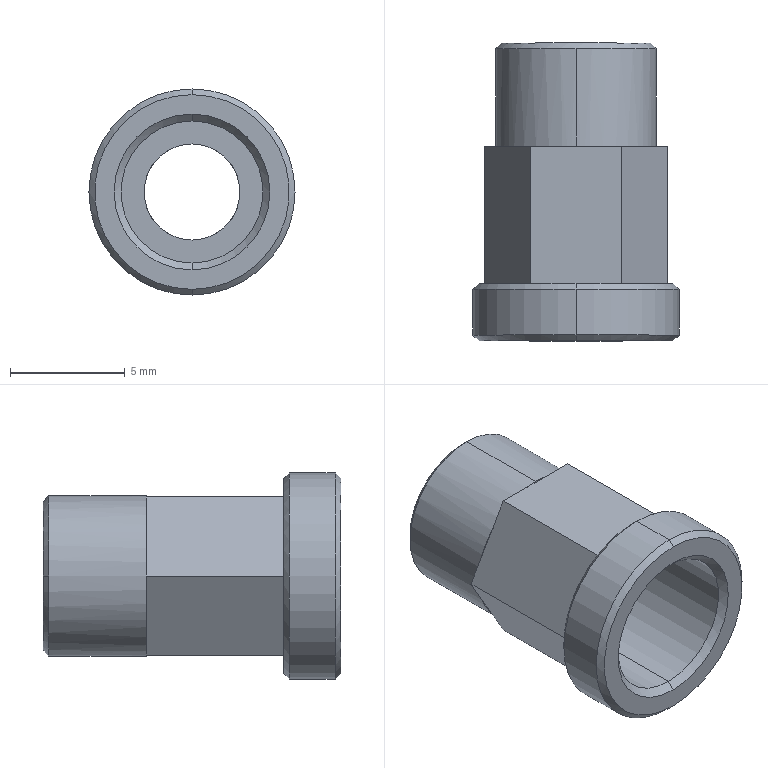Part | NX | features BREP 1 | 1 solid | 40 faces | box 9 x 13 x 9 mm | volume 256.908 mm3 | plane 22 | cone 10 | cylinder 8 | commonest cylinder face diameters 4.2 x2 6.2 x2 7 x2 9 x2
STEP:
#1=CARTESIAN_POINT('',(0.,8.5,3.1));
#2=VERTEX_POINT('',#1);
#3=CARTESIAN_POINT('',(0.,8.5,-3.1));
#4=VERTEX_POINT('',#3);
#5=CARTESIAN_POINT('',(0.,8.5,0.));
#6=DIRECTION('',(0.,-1.,0.));
#7=DIRECTION('',(0.,0.,-1.));
#8=AXIS2_PLACEMENT_3D('',#5,#6,#7);
#9=CIRCLE('',#8,3.1);
#10=EDGE_CURVE('',#2,#4,#9,.T.);
#11=ORIENTED_EDGE('',*,*,#10,.F.);
#12=CARTESIAN_POINT('',(0.,0.3,3.1));
#13=VERTEX_POINT('',#12);
#14=CARTESIAN_POINT('',(0.,0.,3.1));
#15=DIRECTION('',(0.,-1.,0.));
#16=VECTOR('',#15,1000.);
#17=LINE('',#14,#16);
#18=EDGE_CURVE('',#13,#2,#17,.F.);
#19=ORIENTED_EDGE('',*,*,#18,.F.);
#20=CARTESIAN_POINT('',(0.,0.3,-3.1));
#21=VERTEX_POINT('',#20);
#22=CARTESIAN_POINT('',(0.,0.3,0.));
#23=DIRECTION('',(0.,1.,0.));
#24=DIRECTION('',(0.,0.,-1.));
#25=AXIS2_PLACEMENT_3D('',#22,#23,#24);
#26=CIRCLE('',#25,3.1);
#27=EDGE_CURVE('',#21,#13,#26,.T.);
#28=ORIENTED_EDGE('',*,*,#27,.F.);
#29=CARTESIAN_POINT('',(0.,0.,-3.1));
#30=DIRECTION('',(0.,-1.,0.));
#31=VECTOR('',#30,1000.);
#32=LINE('',#29,#31);
#33=EDGE_CURVE('',#21,#4,#32,.F.);
#34=ORIENTED_EDGE('',*,*,#33,.T.);
#35=EDGE_LOOP('',(#11,#19,#28,#34));
#36=FACE_BOUND('',#35,.T.);
#37=CARTESIAN_POINT('',(0.,0.,0.));
#38=DIRECTION('',(0.,-1.,0.));
#39=DIRECTION('',(0.,0.,1.));
#40=AXIS2_PLACEMENT_3D('',#37,#38,#39);
#41=CYLINDRICAL_SURFACE('',#40,3.1);
#42=ADVANCED_FACE('',(#36),#41,.F.);
#43=ORIENTED_EDGE('',*,*,#27,.T.);
#44=CARTESIAN_POINT('',(0.,0.,3.4));
#45=VERTEX_POINT('',#44);
#46=CARTESIAN_POINT('',(0.,0.,3.4));
#47=DIRECTION('',(0.,-0.7071,0.7071));
#48=VECTOR('',#47,1000.);
#49=LINE('',#46,#48);
#50=EDGE_CURVE('',#45,#13,#49,.F.);
#51=ORIENTED_EDGE('',*,*,#50,.F.);
#52=CARTESIAN_POINT('',(0.,0.,-3.4));
#53=VERTEX_POINT('',#52);
#54=CARTESIAN_POINT('',(0.,0.,0.));
#55=DIRECTION('',(0.,1.,0.));
#56=DIRECTION('',(0.,0.,-1.));
#57=AXIS2_PLACEMENT_3D('',#54,#55,#56);
#58=CIRCLE('',#57,3.4);
#59=EDGE_CURVE('',#53,#45,#58,.T.);
#60=ORIENTED_EDGE('',*,*,#59,.F.);
#61=CARTESIAN_POINT('',(0.,0.,-3.4));
#62=DIRECTION('',(0.,-0.7071,-0.7071));
#63=VECTOR('',#62,1000.);
#64=LINE('',#61,#63);
#65=EDGE_CURVE('',#53,#21,#64,.F.);
#66=ORIENTED_EDGE('',*,*,#65,.T.);
#67=EDGE_LOOP('',(#43,#51,#60,#66));
#68=FACE_BOUND('',#67,.T.);
#69=CARTESIAN_POINT('',(0.,0.,0.));
#70=DIRECTION('',(0.,-1.,0.));
#71=DIRECTION('',(0.,0.,1.));
#72=AXIS2_PLACEMENT_3D('',#69,#70,#71);
#73=CONICAL_SURFACE('',#72,3.4,0.7854);
#74=ADVANCED_FACE('',(#68),#73,.F.);
#75=CARTESIAN_POINT('',(0.,8.5,2.1));
#76=VERTEX_POINT('',#75);
#77=CARTESIAN_POINT('',(0.,8.5,-2.1));
#78=VERTEX_POINT('',#77);
#79=CARTESIAN_POINT('',(0.,8.5,0.));
#80=DIRECTION('',(0.,-1.,0.));
#81=DIRECTION('',(0.,0.,1.));
#82=AXIS2_PLACEMENT_3D('',#79,#80,#81);
#83=CIRCLE('',#82,2.1);
#84=EDGE_CURVE('',#76,#78,#83,.T.);
#85=ORIENTED_EDGE('',*,*,#84,.T.);
#86=CARTESIAN_POINT('',(0.,12.75,-2.1));
#87=VERTEX_POINT('',#86);
#88=CARTESIAN_POINT('',(0.,6.95,-2.1));
#89=DIRECTION('',(0.,1.,0.));
#90=VECTOR('',#89,1000.);
#91=LINE('',#88,#90);
#92=EDGE_CURVE('',#78,#87,#91,.T.);
#93=ORIENTED_EDGE('',*,*,#92,.T.);
#94=CARTESIAN_POINT('',(-2.1,12.75,0.));
#95=VERTEX_POINT('',#94);
#96=CARTESIAN_POINT('',(0.,12.75,0.));
#97=DIRECTION('',(0.,-1.,0.));
#98=DIRECTION('',(0.,0.,1.));
#99=AXIS2_PLACEMENT_3D('',#96,#97,#98);
#100=CIRCLE('',#99,2.1);
#101=EDGE_CURVE('',#95,#87,#100,.T.);
#102=ORIENTED_EDGE('',*,*,#101,.F.);
#103=CARTESIAN_POINT('',(0.,12.75,2.1));
#104=VERTEX_POINT('',#103);
#105=CARTESIAN_POINT('',(0.,12.75,0.));
#106=DIRECTION('',(0.,-1.,0.));
#107=DIRECTION('',(0.,0.,1.));
#108=AXIS2_PLACEMENT_3D('',#105,#106,#107);
#109=CIRCLE('',#108,2.1);
#110=EDGE_CURVE('',#104,#95,#109,.T.);
#111=ORIENTED_EDGE('',*,*,#110,.F.);
#112=CARTESIAN_POINT('',(0.,6.95,2.1));
#113=DIRECTION('',(0.,1.,0.));
#114=VECTOR('',#113,1000.);
#115=LINE('',#112,#114);
#116=EDGE_CURVE('',#76,#104,#115,.T.);
#117=ORIENTED_EDGE('',*,*,#116,.F.);
#118=EDGE_LOOP('',(#85,#93,#102,#111,#117));
#119=FACE_BOUND('',#118,.T.);
#120=CARTESIAN_POINT('',(0.,6.95,0.));
#121=DIRECTION('',(0.,1.,0.));
#122=DIRECTION('',(0.,0.,-1.));
#123=AXIS2_PLACEMENT_3D('',#120,#121,#122);
#124=CYLINDRICAL_SURFACE('',#123,2.1);
#125=ADVANCED_FACE('',(#119),#124,.F.);
#126=ORIENTED_EDGE('',*,*,#101,.T.);
#127=CARTESIAN_POINT('',(2.1,12.75,0.));
#128=VERTEX_POINT('',#127);
#129=CARTESIAN_POINT('',(0.,12.75,0.));
#130=DIRECTION('',(0.,-1.,0.));
#131=DIRECTION('',(0.,0.,1.));
#132=AXIS2_PLACEMENT_3D('',#129,#130,#131);
#133=CIRCLE('',#132,2.1);
#134=EDGE_CURVE('',#87,#128,#133,.T.);
#135=ORIENTED_EDGE('',*,*,#134,.T.);
#136=CARTESIAN_POINT('',(2.35,13.,0.));
#137=VERTEX_POINT('',#136);
#138=CARTESIAN_POINT('',(2.35,13.,0.));
#139=DIRECTION('',(0.7071,0.7071,0.));
#140=VECTOR('',#139,1000.);
#141=LINE('',#138,#140);
#142=EDGE_CURVE('',#137,#128,#141,.F.);
#143=ORIENTED_EDGE('',*,*,#142,.F.);
#144=CARTESIAN_POINT('',(-2.35,13.,0.));
#145=VERTEX_POINT('',#144);
#146=CARTESIAN_POINT('',(0.,13.,0.));
#147=DIRECTION('',(0.,-1.,0.));
#148=DIRECTION('',(-1.,0.,0.));
#149=AXIS2_PLACEMENT_3D('',#146,#147,#148);
#150=CIRCLE('',#149,2.35);
#151=EDGE_CURVE('',#145,#137,#150,.T.);
#152=ORIENTED_EDGE('',*,*,#151,.F.);
#153=CARTESIAN_POINT('',(-2.35,13.,0.));
#154=DIRECTION('',(-0.7071,0.7071,0.));
#155=VECTOR('',#154,1000.);
#156=LINE('',#153,#155);
#157=EDGE_CURVE('',#145,#95,#156,.F.);
#158=ORIENTED_EDGE('',*,*,#157,.T.);
#159=EDGE_LOOP('',(#126,#135,#143,#152,#158));
#160=FACE_BOUND('',#159,.T.);
#161=CARTESIAN_POINT('',(0.,13.,0.));
#162=DIRECTION('',(0.,1.,0.));
#163=DIRECTION('',(1.,0.,0.));
#164=AXIS2_PLACEMENT_3D('',#161,#162,#163);
#165=CONICAL_SURFACE('',#164,2.35,0.7854);
#166=ADVANCED_FACE('',(#160),#165,.F.);
#167=CARTESIAN_POINT('',(0.,-0.000000001,-4.25));
#168=VERTEX_POINT('',#167);
#169=CARTESIAN_POINT('',(0.,-0.000000001,4.25));
#170=VERTEX_POINT('',#169);
#171=CARTESIAN_POINT('',(0.,-0.000000001,0.));
#172=DIRECTION('',(0.,-1.,0.));
#173=DIRECTION('',(0.,0.,1.));
#174=AXIS2_PLACEMENT_3D('',#171,#172,#173);
#175=CIRCLE('',#174,4.25);
#176=EDGE_CURVE('',#168,#170,#175,.T.);
#177=ORIENTED_EDGE('',*,*,#176,.F.);
#178=CARTESIAN_POINT('',(0.,0.25,-4.5));
#179=VERTEX_POINT('',#178);
#180=CARTESIAN_POINT('',(0.,0.25,-4.5));
#181=DIRECTION('',(0.,0.7071,-0.7071));
#182=VECTOR('',#181,1000.);
#183=LINE('',#180,#182);
#184=EDGE_CURVE('',#168,#179,#183,.T.);
#185=ORIENTED_EDGE('',*,*,#184,.T.);
#186=CARTESIAN_POINT('',(0.,0.25,4.5));
#187=VERTEX_POINT('',#186);
#188=CARTESIAN_POINT('',(0.,0.25,0.));
#189=DIRECTION('',(0.,-1.,0.));
#190=DIRECTION('',(0.,0.,1.));
#191=AXIS2_PLACEMENT_3D('',#188,#189,#190);
#192=CIRCLE('',#191,4.5);
#193=EDGE_CURVE('',#179,#187,#192,.T.);
#194=ORIENTED_EDGE('',*,*,#193,.T.);
#195=CARTESIAN_POINT('',(0.,0.25,4.5));
#196=DIRECTION('',(0.,0.7071,0.7071));
#197=VECTOR('',#196,1000.);
#198=LINE('',#195,#197);
#199=EDGE_CURVE('',#170,#187,#198,.T.);
#200=ORIENTED_EDGE('',*,*,#199,.F.);
#201=EDGE_LOOP('',(#177,#185,#194,#200));
#202=FACE_BOUND('',#201,.T.);
#203=CARTESIAN_POINT('',(0.,0.25,0.));
#204=DIRECTION('',(0.,1.,0.));
#205=DIRECTION('',(0.,0.,-1.));
#206=AXIS2_PLACEMENT_3D('',#203,#204,#205);
#207=CONICAL_SURFACE('',#206,4.5,0.7854);
#208=ADVANCED_FACE('',(#202),#207,.T.);
#209=CARTESIAN_POINT('',(0.,2.25,-4.5));
#210=VERTEX_POINT('',#209);
#211=CARTESIAN_POINT('',(0.,2.25,4.5));
#212=VERTEX_POINT('',#211);
#213=CARTESIAN_POINT('',(0.,2.25,0.));
#214=DIRECTION('',(0.,-1.,0.));
#215=DIRECTION('',(0.,0.,-1.));
#216=AXIS2_PLACEMENT_3D('',#213,#214,#215);
#217=CIRCLE('',#216,4.5);
#218=EDGE_CURVE('',#210,#212,#217,.T.);
#219=ORIENTED_EDGE('',*,*,#218,.T.);
#220=CARTESIAN_POINT('',(0.,0.5,4.5));
#221=DIRECTION('',(0.,-1.,0.));
#222=VECTOR('',#221,1000.);
#223=LINE('',#220,#222);
#224=EDGE_CURVE('',#187,#212,#223,.F.);
#225=ORIENTED_EDGE('',*,*,#224,.F.);
#226=ORIENTED_EDGE('',*,*,#193,.F.);
#227=CARTESIAN_POINT('',(0.,0.5,-4.5));
#228=DIRECTION('',(0.,-1.,0.));
#229=VECTOR('',#228,1000.);
#230=LINE('',#227,#229);
#231=EDGE_CURVE('',#179,#210,#230,.F.);
#232=ORIENTED_EDGE('',*,*,#231,.T.);
#233=EDGE_LOOP('',(#219,#225,#226,#232));
#234=FACE_BOUND('',#233,.T.);
#235=CARTESIAN_POINT('',(0.,0.5,0.));
#236=DIRECTION('',(0.,-1.,0.));
#237=DIRECTION('',(0.,0.,1.));
#238=AXIS2_PLACEMENT_3D('',#235,#236,#237);
#239=CYLINDRICAL_SURFACE('',#238,4.5);
#240=ADVANCED_FACE('',(#234),#239,.T.);
#241=CARTESIAN_POINT('',(-3.25,13.,0.));
#242=VERTEX_POINT('',#241);
#243=CARTESIAN_POINT('',(3.25,13.,0.));
#244=VERTEX_POINT('',#243);
#245=CARTESIAN_POINT('',(0.,13.,0.));
#246=DIRECTION('',(0.,1.,0.));
#247=DIRECTION('',(1.,0.,0.));
#248=AXIS2_PLACEMENT_3D('',#245,#246,#247);
#249=CIRCLE('',#248,3.25);
#250=EDGE_CURVE('',#242,#244,#249,.T.);
#251=ORIENTED_EDGE('',*,*,#250,.F.);
#252=CARTESIAN_POINT('',(-3.5,12.75,0.));
#253=VERTEX_POINT('',#252);
#254=CARTESIAN_POINT('',(-3.5,12.75,0.));
#255=DIRECTION('',(-0.7071,-0.7071,0.));
#256=VECTOR('',#255,1000.);
#257=LINE('',#254,#256);
#258=EDGE_CURVE('',#242,#253,#257,.T.);
#259=ORIENTED_EDGE('',*,*,#258,.T.);
#260=CARTESIAN_POINT('',(0.,12.75,3.5));
#261=VERTEX_POINT('',#260);
#262=CARTESIAN_POINT('',(0.,12.75,0.));
#263=DIRECTION('',(0.,1.,0.));
#264=DIRECTION('',(0.,0.,-1.));
#265=AXIS2_PLACEMENT_3D('',#262,#263,#264);
#266=CIRCLE('',#265,3.5);
#267=EDGE_CURVE('',#253,#261,#266,.T.);
#268=ORIENTED_EDGE('',*,*,#267,.T.);
#269=CARTESIAN_POINT('',(3.5,12.75,0.));
#270=VERTEX_POINT('',#269);
#271=CARTESIAN_POINT('',(0.,12.75,0.));
#272=DIRECTION('',(0.,1.,0.));
#273=DIRECTION('',(0.,0.,-1.));
#274=AXIS2_PLACEMENT_3D('',#271,#272,#273);
#275=CIRCLE('',#274,3.5);
#276=EDGE_CURVE('',#261,#270,#275,.T.);
#277=ORIENTED_EDGE('',*,*,#276,.T.);
#278=CARTESIAN_POINT('',(3.5,12.75,0.));
#279=DIRECTION('',(0.7071,-0.7071,0.));
#280=VECTOR('',#279,1000.);
#281=LINE('',#278,#280);
#282=EDGE_CURVE('',#244,#270,#281,.T.);
#283=ORIENTED_EDGE('',*,*,#282,.F.);
#284=EDGE_LOOP('',(#251,#259,#268,#277,#283));
#285=FACE_BOUND('',#284,.T.);
#286=CARTESIAN_POINT('',(0.,12.75,0.));
#287=DIRECTION('',(0.,-1.,0.));
#288=DIRECTION('',(-1.,0.,0.));
#289=AXIS2_PLACEMENT_3D('',#286,#287,#288);
#290=CONICAL_SURFACE('',#289,3.5,0.7854);
#291=ADVANCED_FACE('',(#285),#290,.T.);
#292=CARTESIAN_POINT('',(0.,2.5,-4.25));
#293=VERTEX_POINT('',#292);
#294=CARTESIAN_POINT('',(0.,2.5,4.25));
#295=VERTEX_POINT('',#294);
#296=CARTESIAN_POINT('',(0.,2.5,0.));
#297=DIRECTION('',(0.,-1.,0.));
#298=DIRECTION('',(0.,0.,-1.));
#299=AXIS2_PLACEMENT_3D('',#296,#297,#298);
#300=CIRCLE('',#299,4.25);
#301=EDGE_CURVE('',#293,#295,#300,.T.);
#302=ORIENTED_EDGE('',*,*,#301,.T.);
#303=CARTESIAN_POINT('',(0.,2.25,4.5));
#304=DIRECTION('',(0.,-0.7071,0.7071));
#305=VECTOR('',#304,1000.);
#306=LINE('',#303,#305);
#307=EDGE_CURVE('',#212,#295,#306,.F.);
#308=ORIENTED_EDGE('',*,*,#307,.F.);
#309=ORIENTED_EDGE('',*,*,#218,.F.);
#310=CARTESIAN_POINT('',(0.,2.25,-4.5));
#311=DIRECTION('',(0.,-0.7071,-0.7071));
#312=VECTOR('',#311,1000.);
#313=LINE('',#310,#312);
#314=EDGE_CURVE('',#210,#293,#313,.F.);
#315=ORIENTED_EDGE('',*,*,#314,.T.);
#316=EDGE_LOOP('',(#302,#308,#309,#315));
#317=FACE_BOUND('',#316,.T.);
#318=CARTESIAN_POINT('',(0.,2.25,0.));
#319=DIRECTION('',(0.,-1.,0.));
#320=DIRECTION('',(0.,0.,1.));
#321=AXIS2_PLACEMENT_3D('',#318,#319,#320);
#322=CONICAL_SURFACE('',#321,4.5,0.7854);
#323=ADVANCED_FACE('',(#317),#322,.T.);
#324=CARTESIAN_POINT('',(0.5895,8.5,-3.45));
#325=VERTEX_POINT('',#324);
#326=CARTESIAN_POINT('',(0.,8.5,-3.5));
#327=VERTEX_POINT('',#326);
#328=CARTESIAN_POINT('',(0.,8.5,0.));
#329=DIRECTION('',(0.,1.,0.));
#330=DIRECTION('',(0.,0.,1.));
#331=AXIS2_PLACEMENT_3D('',#328,#329,#330);
#332=CIRCLE('',#331,3.5);
#333=EDGE_CURVE('',#325,#327,#332,.T.);
#334=ORIENTED_EDGE('',*,*,#333,.T.);
#335=CARTESIAN_POINT('',(0.,12.75,-3.5));
#336=VERTEX_POINT('',#335);
#337=CARTESIAN_POINT('',(0.,8.5,-3.5));
#338=DIRECTION('',(0.,1.,0.));
#339=VECTOR('',#338,1000.);
#340=LINE('',#337,#339);
#341=EDGE_CURVE('',#327,#336,#340,.T.);
#342=ORIENTED_EDGE('',*,*,#341,.T.);
#343=CARTESIAN_POINT('',(0.,12.75,0.));
#344=DIRECTION('',(0.,1.,0.));
#345=DIRECTION('',(0.,0.,-1.));
#346=AXIS2_PLACEMENT_3D('',#343,#344,#345);
#347=CIRCLE('',#346,3.5);
#348=EDGE_CURVE('',#270,#336,#347,.T.);
#349=ORIENTED_EDGE('',*,*,#348,.F.);
#350=ORIENTED_EDGE('',*,*,#276,.F.);
#351=CARTESIAN_POINT('',(0.,8.5,3.5));
#352=VERTEX_POINT('',#351);
#353=CARTESIAN_POINT('',(0.,8.5,3.5));
#354=DIRECTION('',(0.,1.,0.));
#355=VECTOR('',#354,1000.);
#356=LINE('',#353,#355);
#357=EDGE_CURVE('',#352,#261,#356,.T.);
#358=ORIENTED_EDGE('',*,*,#357,.F.);
#359=CARTESIAN_POINT('',(0.5895,8.5,3.45));
#360=VERTEX_POINT('',#359);
#361=CARTESIAN_POINT('',(0.,8.5,0.));
#362=DIRECTION('',(0.,1.,0.));
#363=DIRECTION('',(0.,0.,1.));
#364=AXIS2_PLACEMENT_3D('',#361,#362,#363);
#365=CIRCLE('',#364,3.5);
#366=EDGE_CURVE('',#352,#360,#365,.T.);
#367=ORIENTED_EDGE('',*,*,#366,.T.);
#368=CARTESIAN_POINT('',(2.693,8.5,2.236));
#369=VERTEX_POINT('',#368);
#370=CARTESIAN_POINT('',(0.,8.5,0.));
#371=DIRECTION('',(0.,1.,0.));
#372=DIRECTION('',(0.,0.,1.));
#373=AXIS2_PLACEMENT_3D('',#370,#371,#372);
#374=CIRCLE('',#373,3.5);
#375=EDGE_CURVE('',#360,#369,#374,.T.);
#376=ORIENTED_EDGE('',*,*,#375,.T.);
#377=CARTESIAN_POINT('',(3.283,8.5,1.214));
#378=VERTEX_POINT('',#377);
#379=CARTESIAN_POINT('',(0.,8.5,0.));
#380=DIRECTION('',(0.,1.,0.));
#381=DIRECTION('',(0.,0.,1.));
#382=AXIS2_PLACEMENT_3D('',#379,#380,#381);
#383=CIRCLE('',#382,3.5);
#384=EDGE_CURVE('',#369,#378,#383,.T.);
#385=ORIENTED_EDGE('',*,*,#384,.T.);
#386=CARTESIAN_POINT('',(3.283,8.5,-1.214));
#387=VERTEX_POINT('',#386);
#388=CARTESIAN_POINT('',(0.,8.5,0.));
#389=DIRECTION('',(0.,1.,0.));
#390=DIRECTION('',(0.,0.,1.));
#391=AXIS2_PLACEMENT_3D('',#388,#389,#390);
#392=CIRCLE('',#391,3.5);
#393=EDGE_CURVE('',#378,#387,#392,.T.);
#394=ORIENTED_EDGE('',*,*,#393,.T.);
#395=CARTESIAN_POINT('',(2.693,8.5,-2.236));
#396=VERTEX_POINT('',#395);
#397=CARTESIAN_POINT('',(0.,8.5,0.));
#398=DIRECTION('',(0.,1.,0.));
#399=DIRECTION('',(0.,0.,1.));
#400=AXIS2_PLACEMENT_3D('',#397,#398,#399);
#401=CIRCLE('',#400,3.5);
#402=EDGE_CURVE('',#387,#396,#401,.T.);
#403=ORIENTED_EDGE('',*,*,#402,.T.);
#404=CARTESIAN_POINT('',(0.,8.5,0.));
#405=DIRECTION('',(0.,1.,0.));
#406=DIRECTION('',(0.,0.,1.));
#407=AXIS2_PLACEMENT_3D('',#404,#405,#406);
#408=CIRCLE('',#407,3.5);
#409=EDGE_CURVE('',#396,#325,#408,.T.);
#410=ORIENTED_EDGE('',*,*,#409,.T.);
#411=EDGE_LOOP('',(#334,#342,#349,#350,#358,#367,#376,#385,#394,#403,#410));
#412=FACE_BOUND('',#411,.T.);
#413=CARTESIAN_POINT('',(0.,8.5,0.));
#414=DIRECTION('',(0.,1.,0.));
#415=DIRECTION('',(0.,0.,-1.));
#416=AXIS2_PLACEMENT_3D('',#413,#414,#415);
#417=CYLINDRICAL_SURFACE('',#416,3.5);
#418=ADVANCED_FACE('',(#412),#417,.T.);
#419=ORIENTED_EDGE('',*,*,#18,.T.);
#420=CARTESIAN_POINT('',(0.,8.5,0.));
#421=DIRECTION('',(0.,-1.,0.));
#422=DIRECTION('',(0.,0.,-1.));
#423=AXIS2_PLACEMENT_3D('',#420,#421,#422);
#424=CIRCLE('',#423,3.1);
#425=EDGE_CURVE('',#4,#2,#424,.T.);
#426=ORIENTED_EDGE('',*,*,#425,.F.);
#427=ORIENTED_EDGE('',*,*,#33,.F.);
#428=CARTESIAN_POINT('',(0.,0.3,0.));
#429=DIRECTION('',(0.,1.,0.));
#430=DIRECTION('',(0.,0.,-1.));
#431=AXIS2_PLACEMENT_3D('',#428,#429,#430);
#432=CIRCLE('',#431,3.1);
#433=EDGE_CURVE('',#13,#21,#432,.T.);
#434=ORIENTED_EDGE('',*,*,#433,.F.);
#435=EDGE_LOOP('',(#419,#426,#427,#434));
#436=FACE_BOUND('',#435,.T.);
#437=CARTESIAN_POINT('',(0.,0.,0.));
#438=DIRECTION('',(0.,-1.,0.));
#439=DIRECTION('',(0.,0.,1.));
#440=AXIS2_PLACEMENT_3D('',#437,#438,#439);
#441=CYLINDRICAL_SURFACE('',#440,3.1);
#442=ADVANCED_FACE('',(#436),#441,.F.);
#443=ORIENTED_EDGE('',*,*,#425,.T.);
#444=ORIENTED_EDGE('',*,*,#10,.T.);
#445=EDGE_LOOP('',(#443,#444));
#446=FACE_BOUND('',#445,.T.);
#447=ORIENTED_EDGE('',*,*,#84,.F.);
#448=CARTESIAN_POINT('',(0.,8.5,0.));
#449=DIRECTION('',(0.,-1.,0.));
#450=DIRECTION('',(0.,0.,1.));
#451=AXIS2_PLACEMENT_3D('',#448,#449,#450);
#452=CIRCLE('',#451,2.1);
#453=EDGE_CURVE('',#78,#76,#452,.T.);
#454=ORIENTED_EDGE('',*,*,#453,.F.);
#455=EDGE_LOOP('',(#447,#454));
#456=FACE_BOUND('',#455,.T.);
#457=CARTESIAN_POINT('',(0.,8.5,0.));
#458=DIRECTION('',(0.,1.,0.));
#459=DIRECTION('',(0.,0.,-1.));
#460=AXIS2_PLACEMENT_3D('',#457,#458,#459);
#461=PLANE('',#460);
#462=ADVANCED_FACE('',(#446,#456),#461,.F.);
#463=ORIENTED_EDGE('',*,*,#50,.T.);
#464=ORIENTED_EDGE('',*,*,#433,.T.);
#465=ORIENTED_EDGE('',*,*,#65,.F.);
#466=CARTESIAN_POINT('',(0.,0.,0.));
#467=DIRECTION('',(0.,1.,0.));
#468=DIRECTION('',(0.,0.,-1.));
#469=AXIS2_PLACEMENT_3D('',#466,#467,#468);
#470=CIRCLE('',#469,3.4);
#471=EDGE_CURVE('',#45,#53,#470,.T.);
#472=ORIENTED_EDGE('',*,*,#471,.F.);
#473=EDGE_LOOP('',(#463,#464,#465,#472));
#474=FACE_BOUND('',#473,.T.);
#475=CARTESIAN_POINT('',(0.,0.,0.));
#476=DIRECTION('',(0.,-1.,0.));
#477=DIRECTION('',(0.,0.,1.));
#478=AXIS2_PLACEMENT_3D('',#475,#476,#477);
#479=CONICAL_SURFACE('',#478,3.4,0.7854);
#480=ADVANCED_FACE('',(#474),#479,.F.);
#481=ORIENTED_EDGE('',*,*,#92,.F.);
#482=ORIENTED_EDGE('',*,*,#453,.T.);
#483=ORIENTED_EDGE('',*,*,#116,.T.);
#484=CARTESIAN_POINT('',(0.,12.75,0.));
#485=DIRECTION('',(0.,-1.,0.));
#486=DIRECTION('',(0.,0.,1.));
#487=AXIS2_PLACEMENT_3D('',#484,#485,#486);
#488=CIRCLE('',#487,2.1);
#489=EDGE_CURVE('',#128,#104,#488,.T.);
#490=ORIENTED_EDGE('',*,*,#489,.F.);
#491=ORIENTED_EDGE('',*,*,#134,.F.);
#492=EDGE_LOOP('',(#481,#482,#483,#490,#491));
#493=FACE_BOUND('',#492,.T.);
#494=CARTESIAN_POINT('',(0.,6.95,0.));
#495=DIRECTION('',(0.,1.,0.));
#496=DIRECTION('',(0.,0.,-1.));
#497=AXIS2_PLACEMENT_3D('',#494,#495,#496);
#498=CYLINDRICAL_SURFACE('',#497,2.1);
#499=ADVANCED_FACE('',(#493),#498,.F.);
#500=CARTESIAN_POINT('',(0.,-0.000000001,0.));
#501=DIRECTION('',(0.,-1.,0.));
#502=DIRECTION('',(0.,0.,1.));
#503=AXIS2_PLACEMENT_3D('',#500,#501,#502);
#504=CIRCLE('',#503,4.25);
#505=EDGE_CURVE('',#170,#168,#504,.T.);
#506=ORIENTED_EDGE('',*,*,#505,.T.);
#507=ORIENTED_EDGE('',*,*,#176,.T.);
#508=EDGE_LOOP('',(#506,#507));
#509=FACE_BOUND('',#508,.T.);
#510=ORIENTED_EDGE('',*,*,#59,.T.);
#511=ORIENTED_EDGE('',*,*,#471,.T.);
#512=EDGE_LOOP('',(#510,#511));
#513=FACE_BOUND('',#512,.T.);
#514=CARTESIAN_POINT('',(0.,0.,0.));
#515=DIRECTION('',(0.,-1.,0.));
#516=DIRECTION('',(0.,0.,1.));
#517=AXIS2_PLACEMENT_3D('',#514,#515,#516);
#518=PLANE('',#517);
#519=ADVANCED_FACE('',(#509,#513),#518,.T.);
#520=ORIENTED_EDGE('',*,*,#142,.T.);
#521=ORIENTED_EDGE('',*,*,#489,.T.);
#522=ORIENTED_EDGE('',*,*,#110,.T.);
#523=ORIENTED_EDGE('',*,*,#157,.F.);
#524=CARTESIAN_POINT('',(0.,13.,0.));
#525=DIRECTION('',(0.,-1.,0.));
#526=DIRECTION('',(-1.,0.,0.));
#527=AXIS2_PLACEMENT_3D('',#524,#525,#526);
#528=CIRCLE('',#527,2.35);
#529=EDGE_CURVE('',#137,#145,#528,.T.);
#530=ORIENTED_EDGE('',*,*,#529,.F.);
#531=EDGE_LOOP('',(#520,#521,#522,#523,#530));
#532=FACE_BOUND('',#531,.T.);
#533=CARTESIAN_POINT('',(0.,13.,0.));
#534=DIRECTION('',(0.,1.,0.));
#535=DIRECTION('',(1.,0.,0.));
#536=AXIS2_PLACEMENT_3D('',#533,#534,#535);
#537=CONICAL_SURFACE('',#536,2.35,0.7854);
#538=ADVANCED_FACE('',(#532),#537,.F.);
#539=ORIENTED_EDGE('',*,*,#184,.F.);
#540=ORIENTED_EDGE('',*,*,#505,.F.);
#541=ORIENTED_EDGE('',*,*,#199,.T.);
#542=CARTESIAN_POINT('',(0.,0.25,0.));
#543=DIRECTION('',(0.,-1.,0.));
#544=DIRECTION('',(0.,0.,1.));
#545=AXIS2_PLACEMENT_3D('',#542,#543,#544);
#546=CIRCLE('',#545,4.5);
#547=EDGE_CURVE('',#187,#179,#546,.T.);
#548=ORIENTED_EDGE('',*,*,#547,.T.);
#549=EDGE_LOOP('',(#539,#540,#541,#548));
#550=FACE_BOUND('',#549,.T.);
#551=CARTESIAN_POINT('',(0.,0.25,0.));
#552=DIRECTION('',(0.,1.,0.));
#553=DIRECTION('',(0.,0.,-1.));
#554=AXIS2_PLACEMENT_3D('',#551,#552,#553);
#555=CONICAL_SURFACE('',#554,4.5,0.7854);
#556=ADVANCED_FACE('',(#550),#555,.T.);
#557=CARTESIAN_POINT('',(0.,13.,0.));
#558=DIRECTION('',(0.,1.,0.));
#559=DIRECTION('',(1.,0.,0.));
#560=AXIS2_PLACEMENT_3D('',#557,#558,#559);
#561=CIRCLE('',#560,3.25);
#562=EDGE_CURVE('',#244,#242,#561,.T.);
#563=ORIENTED_EDGE('',*,*,#562,.T.);
#564=ORIENTED_EDGE('',*,*,#250,.T.);
#565=EDGE_LOOP('',(#563,#564));
#566=FACE_BOUND('',#565,.T.);
#567=ORIENTED_EDGE('',*,*,#151,.T.);
#568=ORIENTED_EDGE('',*,*,#529,.T.);
#569=EDGE_LOOP('',(#567,#568));
#570=FACE_BOUND('',#569,.T.);
#571=CARTESIAN_POINT('',(0.,13.,0.));
#572=DIRECTION('',(0.,1.,0.));
#573=DIRECTION('',(0.,0.,-1.));
#574=AXIS2_PLACEMENT_3D('',#571,#572,#573);
#575=PLANE('',#574);
#576=ADVANCED_FACE('',(#566,#570),#575,.T.);
#577=ORIENTED_EDGE('',*,*,#224,.T.);
#578=CARTESIAN_POINT('',(0.,2.25,0.));
#579=DIRECTION('',(0.,-1.,0.));
#580=DIRECTION('',(0.,0.,-1.));
#581=AXIS2_PLACEMENT_3D('',#578,#579,#580);
#582=CIRCLE('',#581,4.5);
#583=EDGE_CURVE('',#212,#210,#582,.T.);
#584=ORIENTED_EDGE('',*,*,#583,.T.);
#585=ORIENTED_EDGE('',*,*,#231,.F.);
#586=ORIENTED_EDGE('',*,*,#547,.F.);
#587=EDGE_LOOP('',(#577,#584,#585,#586));
#588=FACE_BOUND('',#587,.T.);
#589=CARTESIAN_POINT('',(0.,0.5,0.));
#590=DIRECTION('',(0.,-1.,0.));
#591=DIRECTION('',(0.,0.,1.));
#592=AXIS2_PLACEMENT_3D('',#589,#590,#591);
#593=CYLINDRICAL_SURFACE('',#592,4.5);
#594=ADVANCED_FACE('',(#588),#593,.T.);
#595=ORIENTED_EDGE('',*,*,#258,.F.);
#596=ORIENTED_EDGE('',*,*,#562,.F.);
#597=ORIENTED_EDGE('',*,*,#282,.T.);
#598=ORIENTED_EDGE('',*,*,#348,.T.);
#599=CARTESIAN_POINT('',(0.,12.75,0.));
#600=DIRECTION('',(0.,1.,0.));
#601=DIRECTION('',(0.,0.,-1.));
#602=AXIS2_PLACEMENT_3D('',#599,#600,#601);
#603=CIRCLE('',#602,3.5);
#604=EDGE_CURVE('',#336,#253,#603,.T.);
#605=ORIENTED_EDGE('',*,*,#604,.T.);
#606=EDGE_LOOP('',(#595,#596,#597,#598,#605));
#607=FACE_BOUND('',#606,.T.);
#608=CARTESIAN_POINT('',(0.,12.75,0.));
#609=DIRECTION('',(0.,-1.,0.));
#610=DIRECTION('',(-1.,0.,0.));
#611=AXIS2_PLACEMENT_3D('',#608,#609,#610);
#612=CONICAL_SURFACE('',#611,3.5,0.7854);
#613=ADVANCED_FACE('',(#607),#612,.T.);
#614=ORIENTED_EDGE('',*,*,#307,.T.);
#615=CARTESIAN_POINT('',(0.,2.5,0.));
#616=DIRECTION('',(0.,-1.,0.));
#617=DIRECTION('',(0.,0.,-1.));
#618=AXIS2_PLACEMENT_3D('',#615,#616,#617);
#619=CIRCLE('',#618,4.25);
#620=EDGE_CURVE('',#295,#293,#619,.T.);
#621=ORIENTED_EDGE('',*,*,#620,.T.);
#622=ORIENTED_EDGE('',*,*,#314,.F.);
#623=ORIENTED_EDGE('',*,*,#583,.F.);
#624=EDGE_LOOP('',(#614,#621,#622,#623));
#625=FACE_BOUND('',#624,.T.);
#626=CARTESIAN_POINT('',(0.,2.25,0.));
#627=DIRECTION('',(0.,-1.,0.));
#628=DIRECTION('',(0.,0.,1.));
#629=AXIS2_PLACEMENT_3D('',#626,#627,#628);
#630=CONICAL_SURFACE('',#629,4.5,0.7854);
#631=ADVANCED_FACE('',(#625),#630,.T.);
#632=ORIENTED_EDGE('',*,*,#341,.F.);
#633=CARTESIAN_POINT('',(-0.5895,8.5,-3.45));
#634=VERTEX_POINT('',#633);
#635=CARTESIAN_POINT('',(0.,8.5,0.));
#636=DIRECTION('',(0.,1.,0.));
#637=DIRECTION('',(0.,0.,1.));
#638=AXIS2_PLACEMENT_3D('',#635,#636,#637);
#639=CIRCLE('',#638,3.5);
#640=EDGE_CURVE('',#327,#634,#639,.T.);
#641=ORIENTED_EDGE('',*,*,#640,.T.);
#642=CARTESIAN_POINT('',(-2.693,8.5,-2.236));
#643=VERTEX_POINT('',#642);
#644=CARTESIAN_POINT('',(0.,8.5,0.));
#645=DIRECTION('',(0.,1.,0.));
#646=DIRECTION('',(0.,0.,1.));
#647=AXIS2_PLACEMENT_3D('',#644,#645,#646);
#648=CIRCLE('',#647,3.5);
#649=EDGE_CURVE('',#634,#643,#648,.T.);
#650=ORIENTED_EDGE('',*,*,#649,.T.);
#651=CARTESIAN_POINT('',(-3.283,8.5,-1.214));
#652=VERTEX_POINT('',#651);
#653=CARTESIAN_POINT('',(0.,8.5,0.));
#654=DIRECTION('',(0.,1.,0.));
#655=DIRECTION('',(0.,0.,1.));
#656=AXIS2_PLACEMENT_3D('',#653,#654,#655);
#657=CIRCLE('',#656,3.5);
#658=EDGE_CURVE('',#643,#652,#657,.T.);
#659=ORIENTED_EDGE('',*,*,#658,.T.);
#660=CARTESIAN_POINT('',(-3.283,8.5,1.214));
#661=VERTEX_POINT('',#660);
#662=CARTESIAN_POINT('',(0.,8.5,0.));
#663=DIRECTION('',(0.,1.,0.));
#664=DIRECTION('',(0.,0.,1.));
#665=AXIS2_PLACEMENT_3D('',#662,#663,#664);
#666=CIRCLE('',#665,3.5);
#667=EDGE_CURVE('',#652,#661,#666,.T.);
#668=ORIENTED_EDGE('',*,*,#667,.T.);
#669=CARTESIAN_POINT('',(-2.693,8.5,2.236));
#670=VERTEX_POINT('',#669);
#671=CARTESIAN_POINT('',(0.,8.5,0.));
#672=DIRECTION('',(0.,1.,0.));
#673=DIRECTION('',(0.,0.,1.));
#674=AXIS2_PLACEMENT_3D('',#671,#672,#673);
#675=CIRCLE('',#674,3.5);
#676=EDGE_CURVE('',#661,#670,#675,.T.);
#677=ORIENTED_EDGE('',*,*,#676,.T.);
#678=CARTESIAN_POINT('',(-0.5895,8.5,3.45));
#679=VERTEX_POINT('',#678);
#680=CARTESIAN_POINT('',(0.,8.5,0.));
#681=DIRECTION('',(0.,1.,0.));
#682=DIRECTION('',(0.,0.,1.));
#683=AXIS2_PLACEMENT_3D('',#680,#681,#682);
#684=CIRCLE('',#683,3.5);
#685=EDGE_CURVE('',#670,#679,#684,.T.);
#686=ORIENTED_EDGE('',*,*,#685,.T.);
#687=CARTESIAN_POINT('',(0.,8.5,0.));
#688=DIRECTION('',(0.,1.,0.));
#689=DIRECTION('',(0.,0.,1.));
#690=AXIS2_PLACEMENT_3D('',#687,#688,#689);
#691=CIRCLE('',#690,3.5);
#692=EDGE_CURVE('',#679,#352,#691,.T.);
#693=ORIENTED_EDGE('',*,*,#692,.T.);
#694=ORIENTED_EDGE('',*,*,#357,.T.);
#695=ORIENTED_EDGE('',*,*,#267,.F.);
#696=ORIENTED_EDGE('',*,*,#604,.F.);
#697=EDGE_LOOP('',(#632,#641,#650,#659,#668,#677,#686,#693,#694,#695,#696));
#698=FACE_BOUND('',#697,.T.);
#699=CARTESIAN_POINT('',(0.,8.5,0.));
#700=DIRECTION('',(0.,1.,0.));
#701=DIRECTION('',(0.,0.,-1.));
#702=AXIS2_PLACEMENT_3D('',#699,#700,#701);
#703=CYLINDRICAL_SURFACE('',#702,3.5);
#704=ADVANCED_FACE('',(#698),#703,.T.);
#705=ORIENTED_EDGE('',*,*,#301,.F.);
#706=ORIENTED_EDGE('',*,*,#620,.F.);
#707=EDGE_LOOP('',(#705,#706));
#708=FACE_BOUND('',#707,.T.);
#709=CARTESIAN_POINT('',(1.992,2.5,3.45));
#710=VERTEX_POINT('',#709);
#711=CARTESIAN_POINT('',(-1.992,2.5,3.45));
#712=VERTEX_POINT('',#711);
#713=CARTESIAN_POINT('',(0.,2.5,3.45));
#714=DIRECTION('',(-1.,0.,0.));
#715=VECTOR('',#714,1000.);
#716=LINE('',#713,#715);
#717=EDGE_CURVE('',#710,#712,#716,.T.);
#718=ORIENTED_EDGE('',*,*,#717,.T.);
#719=CARTESIAN_POINT('',(-3.984,2.5,0.));
#720=VERTEX_POINT('',#719);
#721=CARTESIAN_POINT('',(-1.992,2.5,3.45));
#722=DIRECTION('',(-0.5,0.,-0.866));
#723=VECTOR('',#722,1000.);
#724=LINE('',#721,#723);
#725=EDGE_CURVE('',#712,#720,#724,.T.);
#726=ORIENTED_EDGE('',*,*,#725,.T.);
#727=CARTESIAN_POINT('',(-1.992,2.5,-3.45));
#728=VERTEX_POINT('',#727);
#729=CARTESIAN_POINT('',(-3.984,2.5,0.));
#730=DIRECTION('',(0.5,0.,-0.866));
#731=VECTOR('',#730,1000.);
#732=LINE('',#729,#731);
#733=EDGE_CURVE('',#720,#728,#732,.T.);
#734=ORIENTED_EDGE('',*,*,#733,.T.);
#735=CARTESIAN_POINT('',(1.992,2.5,-3.45));
#736=VERTEX_POINT('',#735);
#737=CARTESIAN_POINT('',(0.,2.5,-3.45));
#738=DIRECTION('',(1.,0.,0.));
#739=VECTOR('',#738,1000.);
#740=LINE('',#737,#739);
#741=EDGE_CURVE('',#728,#736,#740,.T.);
#742=ORIENTED_EDGE('',*,*,#741,.T.);
#743=CARTESIAN_POINT('',(3.984,2.5,0.));
#744=VERTEX_POINT('',#743);
#745=CARTESIAN_POINT('',(1.992,2.5,-3.45));
#746=DIRECTION('',(0.5,0.,0.866));
#747=VECTOR('',#746,1000.);
#748=LINE('',#745,#747);
#749=EDGE_CURVE('',#736,#744,#748,.T.);
#750=ORIENTED_EDGE('',*,*,#749,.T.);
#751=CARTESIAN_POINT('',(3.984,2.5,0.));
#752=DIRECTION('',(-0.5,0.,0.866));
#753=VECTOR('',#752,1000.);
#754=LINE('',#751,#753);
#755=EDGE_CURVE('',#744,#710,#754,.T.);
#756=ORIENTED_EDGE('',*,*,#755,.T.);
#757=EDGE_LOOP('',(#718,#726,#734,#742,#750,#756));
#758=FACE_BOUND('',#757,.T.);
#759=CARTESIAN_POINT('',(0.,2.5,0.));
#760=DIRECTION('',(0.,1.,0.));
#761=DIRECTION('',(0.,0.,-1.));
#762=AXIS2_PLACEMENT_3D('',#759,#760,#761);
#763=PLANE('',#762);
#764=ADVANCED_FACE('',(#708,#758),#763,.T.);
#765=CARTESIAN_POINT('',(1.992,8.5,-3.45));
#766=VERTEX_POINT('',#765);
#767=CARTESIAN_POINT('',(2.693,8.5,-2.236));
#768=DIRECTION('',(-0.5,0.,-0.866));
#769=VECTOR('',#768,1000.);
#770=LINE('',#767,#769);
#771=EDGE_CURVE('',#396,#766,#770,.T.);
#772=ORIENTED_EDGE('',*,*,#771,.T.);
#773=CARTESIAN_POINT('',(0.,8.5,-3.45));
#774=DIRECTION('',(-1.,0.,0.));
#775=VECTOR('',#774,1000.);
#776=LINE('',#773,#775);
#777=EDGE_CURVE('',#766,#325,#776,.T.);
#778=ORIENTED_EDGE('',*,*,#777,.T.);
#779=ORIENTED_EDGE('',*,*,#409,.F.);
#780=EDGE_LOOP('',(#772,#778,#779));
#781=FACE_BOUND('',#780,.T.);
#782=CARTESIAN_POINT('',(0.,8.5,0.));
#783=DIRECTION('',(0.,1.,0.));
#784=DIRECTION('',(0.,0.,-1.));
#785=AXIS2_PLACEMENT_3D('',#782,#783,#784);
#786=PLANE('',#785);
#787=ADVANCED_FACE('',(#781),#786,.T.);
#788=ORIENTED_EDGE('',*,*,#402,.F.);
#789=CARTESIAN_POINT('',(2.693,8.5,-2.236));
#790=DIRECTION('',(0.5,0.,0.866));
#791=VECTOR('',#790,1000.);
#792=LINE('',#789,#791);
#793=EDGE_CURVE('',#396,#387,#792,.T.);
#794=ORIENTED_EDGE('',*,*,#793,.F.);
#795=EDGE_LOOP('',(#788,#794));
#796=FACE_BOUND('',#795,.T.);
#797=CARTESIAN_POINT('',(0.,8.5,0.));
#798=DIRECTION('',(0.,1.,0.));
#799=DIRECTION('',(0.,0.,-1.));
#800=AXIS2_PLACEMENT_3D('',#797,#798,#799);
#801=PLANE('',#800);
#802=ADVANCED_FACE('',(#796),#801,.F.);
#803=CARTESIAN_POINT('',(3.984,8.5,0.));
#804=VERTEX_POINT('',#803);
#805=CARTESIAN_POINT('',(3.283,8.5,1.214));
#806=DIRECTION('',(0.5,0.,-0.866));
#807=VECTOR('',#806,1000.);
#808=LINE('',#805,#807);
#809=EDGE_CURVE('',#378,#804,#808,.T.);
#810=ORIENTED_EDGE('',*,*,#809,.T.);
#811=CARTESIAN_POINT('',(3.984,8.5,0.));
#812=DIRECTION('',(-0.5,0.,-0.866));
#813=VECTOR('',#812,1000.);
#814=LINE('',#811,#813);
#815=EDGE_CURVE('',#804,#387,#814,.T.);
#816=ORIENTED_EDGE('',*,*,#815,.T.);
#817=ORIENTED_EDGE('',*,*,#393,.F.);
#818=EDGE_LOOP('',(#810,#816,#817));
#819=FACE_BOUND('',#818,.T.);
#820=CARTESIAN_POINT('',(0.,8.5,0.));
#821=DIRECTION('',(0.,1.,0.));
#822=DIRECTION('',(0.,0.,-1.));
#823=AXIS2_PLACEMENT_3D('',#820,#821,#822);
#824=PLANE('',#823);
#825=ADVANCED_FACE('',(#819),#824,.T.);
#826=ORIENTED_EDGE('',*,*,#384,.F.);
#827=CARTESIAN_POINT('',(3.283,8.5,1.214));
#828=DIRECTION('',(-0.5,0.,0.866));
#829=VECTOR('',#828,1000.);
#830=LINE('',#827,#829);
#831=EDGE_CURVE('',#378,#369,#830,.T.);
#832=ORIENTED_EDGE('',*,*,#831,.F.);
#833=EDGE_LOOP('',(#826,#832));
#834=FACE_BOUND('',#833,.T.);
#835=CARTESIAN_POINT('',(0.,8.5,0.));
#836=DIRECTION('',(0.,1.,0.));
#837=DIRECTION('',(0.,0.,-1.));
#838=AXIS2_PLACEMENT_3D('',#835,#836,#837);
#839=PLANE('',#838);
#840=ADVANCED_FACE('',(#834),#839,.F.);
#841=CARTESIAN_POINT('',(1.992,8.5,3.45));
#842=VERTEX_POINT('',#841);
#843=CARTESIAN_POINT('',(0.,8.5,3.45));
#844=DIRECTION('',(1.,0.,0.));
#845=VECTOR('',#844,1000.);
#846=LINE('',#843,#845);
#847=EDGE_CURVE('',#360,#842,#846,.T.);
#848=ORIENTED_EDGE('',*,*,#847,.T.);
#849=CARTESIAN_POINT('',(1.992,8.5,3.45));
#850=DIRECTION('',(0.5,0.,-0.866));
#851=VECTOR('',#850,1000.);
#852=LINE('',#849,#851);
#853=EDGE_CURVE('',#842,#369,#852,.T.);
#854=ORIENTED_EDGE('',*,*,#853,.T.);
#855=ORIENTED_EDGE('',*,*,#375,.F.);
#856=EDGE_LOOP('',(#848,#854,#855));
#857=FACE_BOUND('',#856,.T.);
#858=CARTESIAN_POINT('',(0.,8.5,0.));
#859=DIRECTION('',(0.,1.,0.));
#860=DIRECTION('',(0.,0.,-1.));
#861=AXIS2_PLACEMENT_3D('',#858,#859,#860);
#862=PLANE('',#861);
#863=ADVANCED_FACE('',(#857),#862,.T.);
#864=ORIENTED_EDGE('',*,*,#692,.F.);
#865=CARTESIAN_POINT('',(0.,8.5,3.45));
#866=DIRECTION('',(-1.,0.,0.));
#867=VECTOR('',#866,1000.);
#868=LINE('',#865,#867);
#869=EDGE_CURVE('',#360,#679,#868,.T.);
#870=ORIENTED_EDGE('',*,*,#869,.F.);
#871=ORIENTED_EDGE('',*,*,#366,.F.);
#872=EDGE_LOOP('',(#864,#870,#871));
#873=FACE_BOUND('',#872,.T.);
#874=CARTESIAN_POINT('',(0.,8.5,0.));
#875=DIRECTION('',(0.,1.,0.));
#876=DIRECTION('',(0.,0.,-1.));
#877=AXIS2_PLACEMENT_3D('',#874,#875,#876);
#878=PLANE('',#877);
#879=ADVANCED_FACE('',(#873),#878,.F.);
#880=CARTESIAN_POINT('',(0.,8.5,-3.45));
#881=DIRECTION('',(1.,0.,0.));
#882=VECTOR('',#881,1000.);
#883=LINE('',#880,#882);
#884=EDGE_CURVE('',#634,#325,#883,.T.);
#885=ORIENTED_EDGE('',*,*,#884,.F.);
#886=ORIENTED_EDGE('',*,*,#640,.F.);
#887=ORIENTED_EDGE('',*,*,#333,.F.);
#888=EDGE_LOOP('',(#885,#886,#887));
#889=FACE_BOUND('',#888,.T.);
#890=CARTESIAN_POINT('',(0.,8.5,0.));
#891=DIRECTION('',(0.,1.,0.));
#892=DIRECTION('',(0.,0.,-1.));
#893=AXIS2_PLACEMENT_3D('',#890,#891,#892);
#894=PLANE('',#893);
#895=ADVANCED_FACE('',(#889),#894,.F.);
#896=CARTESIAN_POINT('',(-1.992,8.5,3.45));
#897=VERTEX_POINT('',#896);
#898=CARTESIAN_POINT('',(-2.693,8.5,2.236));
#899=DIRECTION('',(0.5,0.,0.866));
#900=VECTOR('',#899,1000.);
#901=LINE('',#898,#900);
#902=EDGE_CURVE('',#670,#897,#901,.T.);
#903=ORIENTED_EDGE('',*,*,#902,.T.);
#904=CARTESIAN_POINT('',(0.,8.5,3.45));
#905=DIRECTION('',(1.,0.,0.));
#906=VECTOR('',#905,1000.);
#907=LINE('',#904,#906);
#908=EDGE_CURVE('',#897,#679,#907,.T.);
#909=ORIENTED_EDGE('',*,*,#908,.T.);
#910=ORIENTED_EDGE('',*,*,#685,.F.);
#911=EDGE_LOOP('',(#903,#909,#910));
#912=FACE_BOUND('',#911,.T.);
#913=CARTESIAN_POINT('',(0.,8.5,0.));
#914=DIRECTION('',(0.,1.,0.));
#915=DIRECTION('',(0.,0.,-1.));
#916=AXIS2_PLACEMENT_3D('',#913,#914,#915);
#917=PLANE('',#916);
#918=ADVANCED_FACE('',(#912),#917,.T.);
#919=ORIENTED_EDGE('',*,*,#676,.F.);
#920=CARTESIAN_POINT('',(-2.693,8.5,2.236));
#921=DIRECTION('',(-0.5,0.,-0.866));
#922=VECTOR('',#921,1000.);
#923=LINE('',#920,#922);
#924=EDGE_CURVE('',#670,#661,#923,.T.);
#925=ORIENTED_EDGE('',*,*,#924,.F.);
#926=EDGE_LOOP('',(#919,#925));
#927=FACE_BOUND('',#926,.T.);
#928=CARTESIAN_POINT('',(0.,8.5,0.));
#929=DIRECTION('',(0.,1.,0.));
#930=DIRECTION('',(0.,0.,-1.));
#931=AXIS2_PLACEMENT_3D('',#928,#929,#930);
#932=PLANE('',#931);
#933=ADVANCED_FACE('',(#927),#932,.F.);
#934=CARTESIAN_POINT('',(-3.984,8.5,0.));
#935=VERTEX_POINT('',#934);
#936=CARTESIAN_POINT('',(-3.984,8.5,0.));
#937=DIRECTION('',(0.5,0.,0.866));
#938=VECTOR('',#937,1000.);
#939=LINE('',#936,#938);
#940=EDGE_CURVE('',#935,#661,#939,.T.);
#941=ORIENTED_EDGE('',*,*,#940,.T.);
#942=ORIENTED_EDGE('',*,*,#667,.F.);
#943=CARTESIAN_POINT('',(-3.283,8.5,-1.214));
#944=DIRECTION('',(-0.5,0.,0.866));
#945=VECTOR('',#944,1000.);
#946=LINE('',#943,#945);
#947=EDGE_CURVE('',#652,#935,#946,.T.);
#948=ORIENTED_EDGE('',*,*,#947,.T.);
#949=EDGE_LOOP('',(#941,#942,#948));
#950=FACE_BOUND('',#949,.T.);
#951=CARTESIAN_POINT('',(0.,8.5,0.));
#952=DIRECTION('',(0.,1.,0.));
#953=DIRECTION('',(0.,0.,-1.));
#954=AXIS2_PLACEMENT_3D('',#951,#952,#953);
#955=PLANE('',#954);
#956=ADVANCED_FACE('',(#950),#955,.T.);
#957=ORIENTED_EDGE('',*,*,#658,.F.);
#958=CARTESIAN_POINT('',(-3.283,8.5,-1.214));
#959=DIRECTION('',(0.5,0.,-0.866));
#960=VECTOR('',#959,1000.);
#961=LINE('',#958,#960);
#962=EDGE_CURVE('',#652,#643,#961,.T.);
#963=ORIENTED_EDGE('',*,*,#962,.F.);
#964=EDGE_LOOP('',(#957,#963));
#965=FACE_BOUND('',#964,.T.);
#966=CARTESIAN_POINT('',(0.,8.5,0.));
#967=DIRECTION('',(0.,1.,0.));
#968=DIRECTION('',(0.,0.,-1.));
#969=AXIS2_PLACEMENT_3D('',#966,#967,#968);
#970=PLANE('',#969);
#971=ADVANCED_FACE('',(#965),#970,.F.);
#972=CARTESIAN_POINT('',(-1.992,8.5,-3.45));
#973=VERTEX_POINT('',#972);
#974=CARTESIAN_POINT('',(0.,8.5,-3.45));
#975=DIRECTION('',(-1.,0.,0.));
#976=VECTOR('',#975,1000.);
#977=LINE('',#974,#976);
#978=EDGE_CURVE('',#634,#973,#977,.T.);
#979=ORIENTED_EDGE('',*,*,#978,.T.);
#980=CARTESIAN_POINT('',(-1.992,8.5,-3.45));
#981=DIRECTION('',(-0.5,0.,0.866));
#982=VECTOR('',#981,1000.);
#983=LINE('',#980,#982);
#984=EDGE_CURVE('',#973,#643,#983,.T.);
#985=ORIENTED_EDGE('',*,*,#984,.T.);
#986=ORIENTED_EDGE('',*,*,#649,.F.);
#987=EDGE_LOOP('',(#979,#985,#986));
#988=FACE_BOUND('',#987,.T.);
#989=CARTESIAN_POINT('',(0.,8.5,0.));
#990=DIRECTION('',(0.,1.,0.));
#991=DIRECTION('',(0.,0.,-1.));
#992=AXIS2_PLACEMENT_3D('',#989,#990,#991);
#993=PLANE('',#992);
#994=ADVANCED_FACE('',(#988),#993,.T.);
#995=CARTESIAN_POINT('',(-1.992,2.5,3.45));
#996=DIRECTION('',(0.,1.,0.));
#997=VECTOR('',#996,1000.);
#998=LINE('',#995,#997);
#999=EDGE_CURVE('',#712,#897,#998,.T.);
#1000=ORIENTED_EDGE('',*,*,#999,.T.);
#1001=ORIENTED_EDGE('',*,*,#902,.F.);
#1002=ORIENTED_EDGE('',*,*,#924,.T.);
#1003=ORIENTED_EDGE('',*,*,#940,.F.);
#1004=CARTESIAN_POINT('',(-3.984,2.5,0.));
#1005=DIRECTION('',(0.,-1.,0.));
#1006=VECTOR('',#1005,1000.);
#1007=LINE('',#1004,#1006);
#1008=EDGE_CURVE('',#935,#720,#1007,.T.);
#1009=ORIENTED_EDGE('',*,*,#1008,.T.);
#1010=ORIENTED_EDGE('',*,*,#725,.F.);
#1011=EDGE_LOOP('',(#1000,#1001,#1002,#1003,#1009,#1010));
#1012=FACE_BOUND('',#1011,.T.);
#1013=CARTESIAN_POINT('',(-3.984,2.5,0.));
#1014=DIRECTION('',(-0.866,0.,0.5));
#1015=DIRECTION('',(-0.5,0.,-0.866));
#1016=AXIS2_PLACEMENT_3D('',#1013,#1014,#1015);
#1017=PLANE('',#1016);
#1018=ADVANCED_FACE('',(#1012),#1017,.T.);
#1019=CARTESIAN_POINT('',(1.992,2.5,3.45));
#1020=DIRECTION('',(0.,1.,0.));
#1021=VECTOR('',#1020,1000.);
#1022=LINE('',#1019,#1021);
#1023=EDGE_CURVE('',#710,#842,#1022,.T.);
#1024=ORIENTED_EDGE('',*,*,#1023,.T.);
#1025=ORIENTED_EDGE('',*,*,#847,.F.);
#1026=ORIENTED_EDGE('',*,*,#869,.T.);
#1027=ORIENTED_EDGE('',*,*,#908,.F.);
#1028=ORIENTED_EDGE('',*,*,#999,.F.);
#1029=ORIENTED_EDGE('',*,*,#717,.F.);
#1030=EDGE_LOOP('',(#1024,#1025,#1026,#1027,#1028,#1029));
#1031=FACE_BOUND('',#1030,.T.);
#1032=CARTESIAN_POINT('',(-1.992,2.5,3.45));
#1033=DIRECTION('',(0.,0.,1.));
#1034=DIRECTION('',(-1.,0.,0.));
#1035=AXIS2_PLACEMENT_3D('',#1032,#1033,#1034);
#1036=PLANE('',#1035);
#1037=ADVANCED_FACE('',(#1031),#1036,.T.);
#1038=CARTESIAN_POINT('',(3.984,2.5,0.));
#1039=DIRECTION('',(0.,1.,0.));
#1040=VECTOR('',#1039,1000.);
#1041=LINE('',#1038,#1040);
#1042=EDGE_CURVE('',#744,#804,#1041,.T.);
#1043=ORIENTED_EDGE('',*,*,#1042,.T.);
#1044=ORIENTED_EDGE('',*,*,#809,.F.);
#1045=ORIENTED_EDGE('',*,*,#831,.T.);
#1046=ORIENTED_EDGE('',*,*,#853,.F.);
#1047=ORIENTED_EDGE('',*,*,#1023,.F.);
#1048=ORIENTED_EDGE('',*,*,#755,.F.);
#1049=EDGE_LOOP('',(#1043,#1044,#1045,#1046,#1047,#1048));
#1050=FACE_BOUND('',#1049,.T.);
#1051=CARTESIAN_POINT('',(1.992,2.5,3.45));
#1052=DIRECTION('',(0.866,0.,0.5));
#1053=DIRECTION('',(-0.5,0.,0.866));
#1054=AXIS2_PLACEMENT_3D('',#1051,#1052,#1053);
#1055=PLANE('',#1054);
#1056=ADVANCED_FACE('',(#1050),#1055,.T.);
#1057=CARTESIAN_POINT('',(1.992,2.5,-3.45));
#1058=DIRECTION('',(0.,1.,0.));
#1059=VECTOR('',#1058,1000.);
#1060=LINE('',#1057,#1059);
#1061=EDGE_CURVE('',#736,#766,#1060,.T.);
#1062=ORIENTED_EDGE('',*,*,#1061,.T.);
#1063=ORIENTED_EDGE('',*,*,#771,.F.);
#1064=ORIENTED_EDGE('',*,*,#793,.T.);
#1065=ORIENTED_EDGE('',*,*,#815,.F.);
#1066=ORIENTED_EDGE('',*,*,#1042,.F.);
#1067=ORIENTED_EDGE('',*,*,#749,.F.);
#1068=EDGE_LOOP('',(#1062,#1063,#1064,#1065,#1066,#1067));
#1069=FACE_BOUND('',#1068,.T.);
#1070=CARTESIAN_POINT('',(3.984,2.5,0.));
#1071=DIRECTION('',(0.866,0.,-0.5));
#1072=DIRECTION('',(0.5,0.,0.866));
#1073=AXIS2_PLACEMENT_3D('',#1070,#1071,#1072);
#1074=PLANE('',#1073);
#1075=ADVANCED_FACE('',(#1069),#1074,.T.);
#1076=CARTESIAN_POINT('',(-1.992,2.5,-3.45));
#1077=DIRECTION('',(0.,1.,0.));
#1078=VECTOR('',#1077,1000.);
#1079=LINE('',#1076,#1078);
#1080=EDGE_CURVE('',#728,#973,#1079,.T.);
#1081=ORIENTED_EDGE('',*,*,#1080,.T.);
#1082=ORIENTED_EDGE('',*,*,#978,.F.);
#1083=ORIENTED_EDGE('',*,*,#884,.T.);
#1084=ORIENTED_EDGE('',*,*,#777,.F.);
#1085=ORIENTED_EDGE('',*,*,#1061,.F.);
#1086=ORIENTED_EDGE('',*,*,#741,.F.);
#1087=EDGE_LOOP('',(#1081,#1082,#1083,#1084,#1085,#1086));
#1088=FACE_BOUND('',#1087,.T.);
#1089=CARTESIAN_POINT('',(1.992,2.5,-3.45));
#1090=DIRECTION('',(0.,0.,-1.));
#1091=DIRECTION('',(1.,0.,0.));
#1092=AXIS2_PLACEMENT_3D('',#1089,#1090,#1091);
#1093=PLANE('',#1092);
#1094=ADVANCED_FACE('',(#1088),#1093,.T.);
#1095=ORIENTED_EDGE('',*,*,#1008,.F.);
#1096=ORIENTED_EDGE('',*,*,#947,.F.);
#1097=ORIENTED_EDGE('',*,*,#962,.T.);
#1098=ORIENTED_EDGE('',*,*,#984,.F.);
#1099=ORIENTED_EDGE('',*,*,#1080,.F.);
#1100=ORIENTED_EDGE('',*,*,#733,.F.);
#1101=EDGE_LOOP('',(#1095,#1096,#1097,#1098,#1099,#1100));
#1102=FACE_BOUND('',#1101,.T.);
#1103=CARTESIAN_POINT('',(-1.992,2.5,-3.45));
#1104=DIRECTION('',(-0.866,0.,-0.5));
#1105=DIRECTION('',(0.5,0.,-0.866));
#1106=AXIS2_PLACEMENT_3D('',#1103,#1104,#1105);
#1107=PLANE('',#1106);
#1108=ADVANCED_FACE('',(#1102),#1107,.T.);
#1109=CLOSED_SHELL('',(#42,#74,#125,#166,#208,#240,#291,#323,#418,#442,#462,#480,#499,#519,#538,#556,#576,#594,#613,#631,#704,#764,#787,#802,#825,#840,#863,#879,#895,#918,#933,#956,#971,#994,#1018,#1037,#1056,#1075,#1094,#1108));
#1110=MANIFOLD_SOLID_BREP('',#1109);
#1111=(LENGTH_UNIT()NAMED_UNIT(*)SI_UNIT(.MILLI.,.METRE.));
#1112=UNCERTAINTY_MEASURE_WITH_UNIT(LENGTH_MEASURE(0.00001),#1111,'','');
#1113=(NAMED_UNIT(*)PLANE_ANGLE_UNIT()SI_UNIT($,.RADIAN.));
#1114=(NAMED_UNIT(*)SI_UNIT($,.STERADIAN.)SOLID_ANGLE_UNIT());
#1115=(GEOMETRIC_REPRESENTATION_CONTEXT(3)GLOBAL_UNCERTAINTY_ASSIGNED_CONTEXT((#1112))GLOBAL_UNIT_ASSIGNED_CONTEXT((#1111,#1113,#1114))REPRESENTATION_CONTEXT('',''));
#1116=ADVANCED_BREP_SHAPE_REPRESENTATION('',(#1110),#1115);